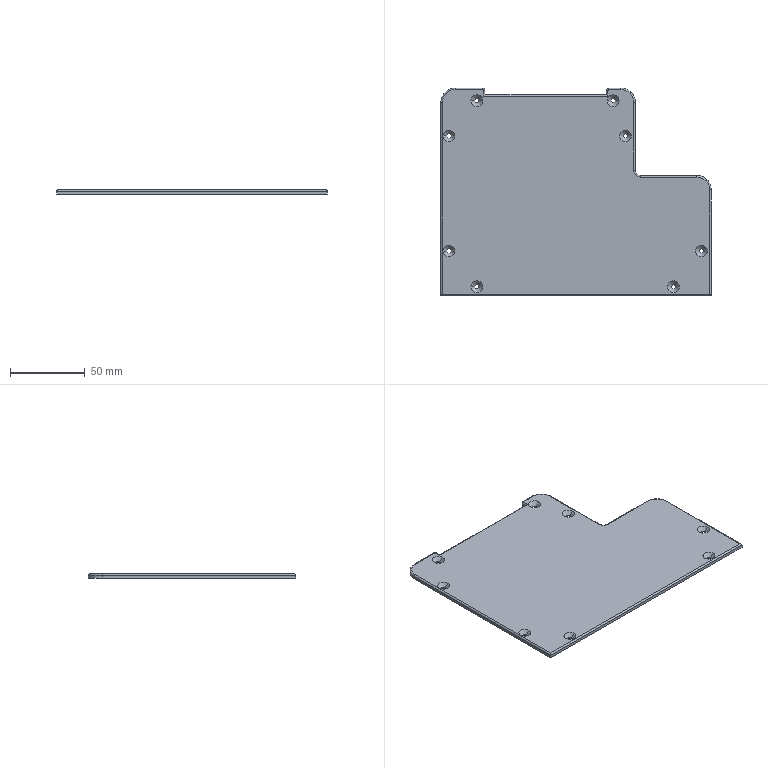Part | STEP file | ASND-0110-SDS_1 | 1 solid | 69 faces | box 181 x 139 x 3 mm | volume 64643 mm3 | cylinder 32 | cone 16 | plane 12 | torus 6 | other 3 | commonest cylinder face diameters 3 x18 2 x10 19.2 x3 7.2 x1